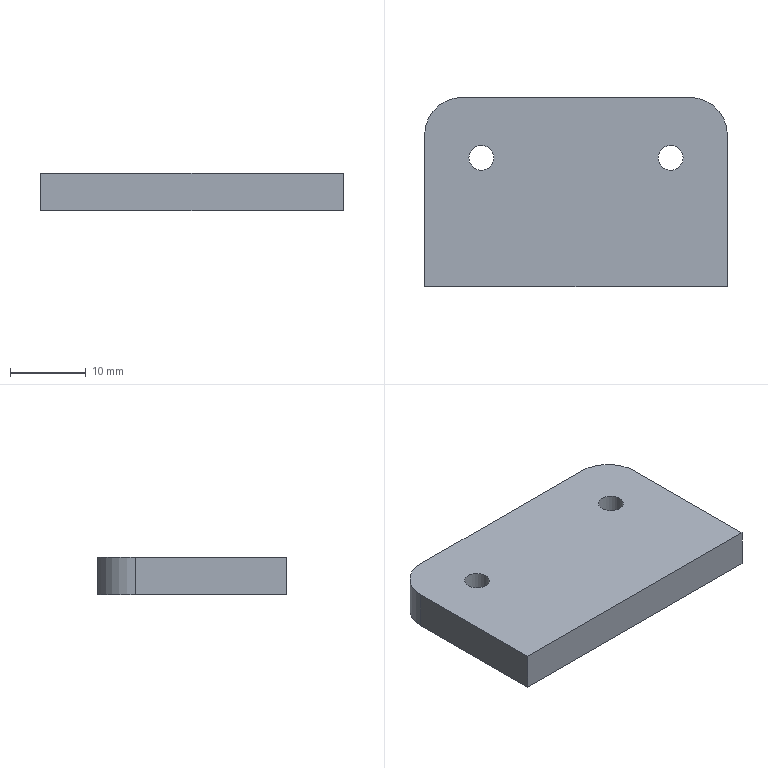Part | NX | features BREP 1 | 1 solid | 10 faces | box 40 x 25 x 5 mm | volume 4861 mm3 | plane 6 | cylinder 4 | commonest cylinder face diameters 3.3 x2 10 x2
STEP:
#1=CARTESIAN_POINT('',(14.15,4.5,5.));
#2=VERTEX_POINT('',#1);
#3=CARTESIAN_POINT('',(12.5,4.5,5.));
#4=DIRECTION('',(0.,0.,1.));
#5=DIRECTION('',(1.,0.,0.));
#6=AXIS2_PLACEMENT_3D('',#3,#4,#5);
#7=CIRCLE('',#6,1.65);
#8=EDGE_CURVE('',#2,#2,#7,.T.);
#9=ORIENTED_EDGE('',*,*,#8,.T.);
#10=EDGE_LOOP('',(#9));
#11=FACE_BOUND('',#10,.T.);
#12=CARTESIAN_POINT('',(14.15,4.5,0.));
#13=VERTEX_POINT('',#12);
#14=CARTESIAN_POINT('',(12.5,4.5,0.));
#15=DIRECTION('',(0.,0.,1.));
#16=DIRECTION('',(1.,0.,0.));
#17=AXIS2_PLACEMENT_3D('',#14,#15,#16);
#18=CIRCLE('',#17,1.65);
#19=EDGE_CURVE('',#13,#13,#18,.T.);
#20=ORIENTED_EDGE('',*,*,#19,.F.);
#21=EDGE_LOOP('',(#20));
#22=FACE_BOUND('',#21,.T.);
#23=CARTESIAN_POINT('',(12.5,4.5,5.));
#24=DIRECTION('',(0.,0.,1.));
#25=DIRECTION('',(1.,0.,0.));
#26=AXIS2_PLACEMENT_3D('',#23,#24,#25);
#27=CYLINDRICAL_SURFACE('',#26,1.65);
#28=ADVANCED_FACE('',(#11,#22),#27,.F.);
#29=CARTESIAN_POINT('',(-10.85,4.5,5.));
#30=VERTEX_POINT('',#29);
#31=CARTESIAN_POINT('',(-12.5,4.5,5.));
#32=DIRECTION('',(0.,0.,1.));
#33=DIRECTION('',(1.,0.,0.));
#34=AXIS2_PLACEMENT_3D('',#31,#32,#33);
#35=CIRCLE('',#34,1.65);
#36=EDGE_CURVE('',#30,#30,#35,.T.);
#37=ORIENTED_EDGE('',*,*,#36,.T.);
#38=EDGE_LOOP('',(#37));
#39=FACE_BOUND('',#38,.T.);
#40=CARTESIAN_POINT('',(-10.85,4.5,0.));
#41=VERTEX_POINT('',#40);
#42=CARTESIAN_POINT('',(-12.5,4.5,0.));
#43=DIRECTION('',(0.,0.,1.));
#44=DIRECTION('',(1.,0.,0.));
#45=AXIS2_PLACEMENT_3D('',#42,#43,#44);
#46=CIRCLE('',#45,1.65);
#47=EDGE_CURVE('',#41,#41,#46,.T.);
#48=ORIENTED_EDGE('',*,*,#47,.F.);
#49=EDGE_LOOP('',(#48));
#50=FACE_BOUND('',#49,.T.);
#51=CARTESIAN_POINT('',(-12.5,4.5,5.));
#52=DIRECTION('',(0.,0.,1.));
#53=DIRECTION('',(1.,0.,0.));
#54=AXIS2_PLACEMENT_3D('',#51,#52,#53);
#55=CYLINDRICAL_SURFACE('',#54,1.65);
#56=ADVANCED_FACE('',(#39,#50),#55,.F.);
#57=CARTESIAN_POINT('',(20.,-12.5,0.));
#58=VERTEX_POINT('',#57);
#59=CARTESIAN_POINT('',(20.,7.5,0.));
#60=VERTEX_POINT('',#59);
#61=CARTESIAN_POINT('',(20.,12.5,0.));
#62=DIRECTION('',(0.,1.,0.));
#63=VECTOR('',#62,1000.);
#64=LINE('',#61,#63);
#65=EDGE_CURVE('',#58,#60,#64,.T.);
#66=ORIENTED_EDGE('',*,*,#65,.T.);
#67=CARTESIAN_POINT('',(20.,7.5,5.));
#68=VERTEX_POINT('',#67);
#69=CARTESIAN_POINT('',(20.,7.5,5.));
#70=DIRECTION('',(0.,0.,1.));
#71=VECTOR('',#70,1000.);
#72=LINE('',#69,#71);
#73=EDGE_CURVE('',#60,#68,#72,.T.);
#74=ORIENTED_EDGE('',*,*,#73,.T.);
#75=CARTESIAN_POINT('',(20.,-12.5,5.));
#76=VERTEX_POINT('',#75);
#77=CARTESIAN_POINT('',(20.,12.5,5.));
#78=DIRECTION('',(0.,1.,0.));
#79=VECTOR('',#78,1000.);
#80=LINE('',#77,#79);
#81=EDGE_CURVE('',#76,#68,#80,.T.);
#82=ORIENTED_EDGE('',*,*,#81,.F.);
#83=CARTESIAN_POINT('',(20.,-12.5,5.));
#84=DIRECTION('',(0.,0.,-1.));
#85=VECTOR('',#84,1000.);
#86=LINE('',#83,#85);
#87=EDGE_CURVE('',#76,#58,#86,.T.);
#88=ORIENTED_EDGE('',*,*,#87,.T.);
#89=EDGE_LOOP('',(#66,#74,#82,#88));
#90=FACE_BOUND('',#89,.T.);
#91=CARTESIAN_POINT('',(20.,12.5,5.));
#92=DIRECTION('',(-1.,0.,0.));
#93=DIRECTION('',(0.,-1.,0.));
#94=AXIS2_PLACEMENT_3D('',#91,#92,#93);
#95=PLANE('',#94);
#96=ADVANCED_FACE('',(#90),#95,.F.);
#97=CARTESIAN_POINT('',(15.,12.5,0.));
#98=VERTEX_POINT('',#97);
#99=CARTESIAN_POINT('',(-15.,12.5,0.));
#100=VERTEX_POINT('',#99);
#101=CARTESIAN_POINT('',(-20.,12.5,0.));
#102=DIRECTION('',(-1.,0.,0.));
#103=VECTOR('',#102,1000.);
#104=LINE('',#101,#103);
#105=EDGE_CURVE('',#98,#100,#104,.T.);
#106=ORIENTED_EDGE('',*,*,#105,.T.);
#107=CARTESIAN_POINT('',(-15.,12.5,5.));
#108=VERTEX_POINT('',#107);
#109=CARTESIAN_POINT('',(-15.,12.5,5.));
#110=DIRECTION('',(0.,0.,1.));
#111=VECTOR('',#110,1000.);
#112=LINE('',#109,#111);
#113=EDGE_CURVE('',#100,#108,#112,.T.);
#114=ORIENTED_EDGE('',*,*,#113,.T.);
#115=CARTESIAN_POINT('',(15.,12.5,5.));
#116=VERTEX_POINT('',#115);
#117=CARTESIAN_POINT('',(-20.,12.5,5.));
#118=DIRECTION('',(-1.,0.,0.));
#119=VECTOR('',#118,1000.);
#120=LINE('',#117,#119);
#121=EDGE_CURVE('',#116,#108,#120,.T.);
#122=ORIENTED_EDGE('',*,*,#121,.F.);
#123=CARTESIAN_POINT('',(15.,12.5,5.));
#124=DIRECTION('',(0.,0.,-1.));
#125=VECTOR('',#124,1000.);
#126=LINE('',#123,#125);
#127=EDGE_CURVE('',#116,#98,#126,.T.);
#128=ORIENTED_EDGE('',*,*,#127,.T.);
#129=EDGE_LOOP('',(#106,#114,#122,#128));
#130=FACE_BOUND('',#129,.T.);
#131=CARTESIAN_POINT('',(-20.,12.5,5.));
#132=DIRECTION('',(0.,-1.,0.));
#133=DIRECTION('',(0.,0.,-1.));
#134=AXIS2_PLACEMENT_3D('',#131,#132,#133);
#135=PLANE('',#134);
#136=ADVANCED_FACE('',(#130),#135,.F.);
#137=CARTESIAN_POINT('',(-20.,7.5,5.));
#138=VERTEX_POINT('',#137);
#139=CARTESIAN_POINT('',(-20.,-12.5,5.));
#140=VERTEX_POINT('',#139);
#141=CARTESIAN_POINT('',(-20.,12.5,5.));
#142=DIRECTION('',(0.,-1.,0.));
#143=VECTOR('',#142,1000.);
#144=LINE('',#141,#143);
#145=EDGE_CURVE('',#138,#140,#144,.T.);
#146=ORIENTED_EDGE('',*,*,#145,.F.);
#147=CARTESIAN_POINT('',(-20.,7.5,0.));
#148=VERTEX_POINT('',#147);
#149=CARTESIAN_POINT('',(-20.,7.5,5.));
#150=DIRECTION('',(0.,0.,-1.));
#151=VECTOR('',#150,1000.);
#152=LINE('',#149,#151);
#153=EDGE_CURVE('',#138,#148,#152,.T.);
#154=ORIENTED_EDGE('',*,*,#153,.T.);
#155=CARTESIAN_POINT('',(-20.,-12.5,0.));
#156=VERTEX_POINT('',#155);
#157=CARTESIAN_POINT('',(-20.,12.5,0.));
#158=DIRECTION('',(0.,-1.,0.));
#159=VECTOR('',#158,1000.);
#160=LINE('',#157,#159);
#161=EDGE_CURVE('',#148,#156,#160,.T.);
#162=ORIENTED_EDGE('',*,*,#161,.T.);
#163=CARTESIAN_POINT('',(-20.,-12.5,5.));
#164=DIRECTION('',(0.,0.,-1.));
#165=VECTOR('',#164,1000.);
#166=LINE('',#163,#165);
#167=EDGE_CURVE('',#140,#156,#166,.T.);
#168=ORIENTED_EDGE('',*,*,#167,.F.);
#169=EDGE_LOOP('',(#146,#154,#162,#168));
#170=FACE_BOUND('',#169,.T.);
#171=CARTESIAN_POINT('',(-20.,12.5,5.));
#172=DIRECTION('',(1.,0.,0.));
#173=DIRECTION('',(0.,1.,0.));
#174=AXIS2_PLACEMENT_3D('',#171,#172,#173);
#175=PLANE('',#174);
#176=ADVANCED_FACE('',(#170),#175,.F.);
#177=CARTESIAN_POINT('',(-20.,-12.5,0.));
#178=DIRECTION('',(1.,0.,0.));
#179=VECTOR('',#178,1000.);
#180=LINE('',#177,#179);
#181=EDGE_CURVE('',#156,#58,#180,.T.);
#182=ORIENTED_EDGE('',*,*,#181,.T.);
#183=ORIENTED_EDGE('',*,*,#87,.F.);
#184=CARTESIAN_POINT('',(-20.,-12.5,5.));
#185=DIRECTION('',(1.,0.,0.));
#186=VECTOR('',#185,1000.);
#187=LINE('',#184,#186);
#188=EDGE_CURVE('',#140,#76,#187,.T.);
#189=ORIENTED_EDGE('',*,*,#188,.F.);
#190=ORIENTED_EDGE('',*,*,#167,.T.);
#191=EDGE_LOOP('',(#182,#183,#189,#190));
#192=FACE_BOUND('',#191,.T.);
#193=CARTESIAN_POINT('',(-20.,-12.5,5.));
#194=DIRECTION('',(0.,1.,0.));
#195=DIRECTION('',(0.,0.,1.));
#196=AXIS2_PLACEMENT_3D('',#193,#194,#195);
#197=PLANE('',#196);
#198=ADVANCED_FACE('',(#192),#197,.F.);
#199=ORIENTED_EDGE('',*,*,#8,.F.);
#200=EDGE_LOOP('',(#199));
#201=FACE_BOUND('',#200,.T.);
#202=ORIENTED_EDGE('',*,*,#36,.F.);
#203=EDGE_LOOP('',(#202));
#204=FACE_BOUND('',#203,.T.);
#205=ORIENTED_EDGE('',*,*,#121,.T.);
#206=CARTESIAN_POINT('',(-15.,7.5,5.));
#207=DIRECTION('',(0.,0.,1.));
#208=DIRECTION('',(1.,0.,0.));
#209=AXIS2_PLACEMENT_3D('',#206,#207,#208);
#210=CIRCLE('',#209,5.);
#211=EDGE_CURVE('',#108,#138,#210,.T.);
#212=ORIENTED_EDGE('',*,*,#211,.T.);
#213=ORIENTED_EDGE('',*,*,#145,.T.);
#214=ORIENTED_EDGE('',*,*,#188,.T.);
#215=ORIENTED_EDGE('',*,*,#81,.T.);
#216=CARTESIAN_POINT('',(15.,7.5,5.));
#217=DIRECTION('',(0.,0.,1.));
#218=DIRECTION('',(1.,0.,0.));
#219=AXIS2_PLACEMENT_3D('',#216,#217,#218);
#220=CIRCLE('',#219,5.);
#221=EDGE_CURVE('',#68,#116,#220,.T.);
#222=ORIENTED_EDGE('',*,*,#221,.T.);
#223=EDGE_LOOP('',(#205,#212,#213,#214,#215,#222));
#224=FACE_BOUND('',#223,.T.);
#225=CARTESIAN_POINT('',(0.,0.,5.));
#226=DIRECTION('',(0.,0.,1.));
#227=DIRECTION('',(1.,0.,0.));
#228=AXIS2_PLACEMENT_3D('',#225,#226,#227);
#229=PLANE('',#228);
#230=ADVANCED_FACE('',(#201,#204,#224),#229,.T.);
#231=ORIENTED_EDGE('',*,*,#19,.T.);
#232=EDGE_LOOP('',(#231));
#233=FACE_BOUND('',#232,.T.);
#234=ORIENTED_EDGE('',*,*,#47,.T.);
#235=EDGE_LOOP('',(#234));
#236=FACE_BOUND('',#235,.T.);
#237=ORIENTED_EDGE('',*,*,#161,.F.);
#238=CARTESIAN_POINT('',(-15.,7.5,0.));
#239=DIRECTION('',(0.,0.,-1.));
#240=DIRECTION('',(1.,0.,0.));
#241=AXIS2_PLACEMENT_3D('',#238,#239,#240);
#242=CIRCLE('',#241,5.);
#243=EDGE_CURVE('',#148,#100,#242,.T.);
#244=ORIENTED_EDGE('',*,*,#243,.T.);
#245=ORIENTED_EDGE('',*,*,#105,.F.);
#246=CARTESIAN_POINT('',(15.,7.5,0.));
#247=DIRECTION('',(0.,0.,-1.));
#248=DIRECTION('',(1.,0.,0.));
#249=AXIS2_PLACEMENT_3D('',#246,#247,#248);
#250=CIRCLE('',#249,5.);
#251=EDGE_CURVE('',#98,#60,#250,.T.);
#252=ORIENTED_EDGE('',*,*,#251,.T.);
#253=ORIENTED_EDGE('',*,*,#65,.F.);
#254=ORIENTED_EDGE('',*,*,#181,.F.);
#255=EDGE_LOOP('',(#237,#244,#245,#252,#253,#254));
#256=FACE_BOUND('',#255,.T.);
#257=CARTESIAN_POINT('',(0.,0.,0.));
#258=DIRECTION('',(0.,0.,1.));
#259=DIRECTION('',(1.,0.,0.));
#260=AXIS2_PLACEMENT_3D('',#257,#258,#259);
#261=PLANE('',#260);
#262=ADVANCED_FACE('',(#233,#236,#256),#261,.F.);
#263=ORIENTED_EDGE('',*,*,#211,.F.);
#264=ORIENTED_EDGE('',*,*,#113,.F.);
#265=ORIENTED_EDGE('',*,*,#243,.F.);
#266=ORIENTED_EDGE('',*,*,#153,.F.);
#267=EDGE_LOOP('',(#263,#264,#265,#266));
#268=FACE_BOUND('',#267,.T.);
#269=CARTESIAN_POINT('',(-15.,7.5,5.));
#270=DIRECTION('',(0.,0.,-1.));
#271=DIRECTION('',(-1.,0.,0.));
#272=AXIS2_PLACEMENT_3D('',#269,#270,#271);
#273=CYLINDRICAL_SURFACE('',#272,5.);
#274=ADVANCED_FACE('',(#268),#273,.T.);
#275=ORIENTED_EDGE('',*,*,#221,.F.);
#276=ORIENTED_EDGE('',*,*,#73,.F.);
#277=ORIENTED_EDGE('',*,*,#251,.F.);
#278=ORIENTED_EDGE('',*,*,#127,.F.);
#279=EDGE_LOOP('',(#275,#276,#277,#278));
#280=FACE_BOUND('',#279,.T.);
#281=CARTESIAN_POINT('',(15.,7.5,5.));
#282=DIRECTION('',(0.,0.,-1.));
#283=DIRECTION('',(-1.,0.,0.));
#284=AXIS2_PLACEMENT_3D('',#281,#282,#283);
#285=CYLINDRICAL_SURFACE('',#284,5.);
#286=ADVANCED_FACE('',(#280),#285,.T.);
#287=CLOSED_SHELL('',(#28,#56,#96,#136,#176,#198,#230,#262,#274,#286));
#288=MANIFOLD_SOLID_BREP('',#287);
#289=(LENGTH_UNIT()NAMED_UNIT(*)SI_UNIT(.MILLI.,.METRE.));
#290=UNCERTAINTY_MEASURE_WITH_UNIT(LENGTH_MEASURE(0.00001),#289,'','');
#291=(NAMED_UNIT(*)PLANE_ANGLE_UNIT()SI_UNIT($,.RADIAN.));
#292=(NAMED_UNIT(*)SI_UNIT($,.STERADIAN.)SOLID_ANGLE_UNIT());
#293=(GEOMETRIC_REPRESENTATION_CONTEXT(3)GLOBAL_UNCERTAINTY_ASSIGNED_CONTEXT((#290))GLOBAL_UNIT_ASSIGNED_CONTEXT((#289,#291,#292))REPRESENTATION_CONTEXT('',''));
#294=ADVANCED_BREP_SHAPE_REPRESENTATION('',(#288),#293);